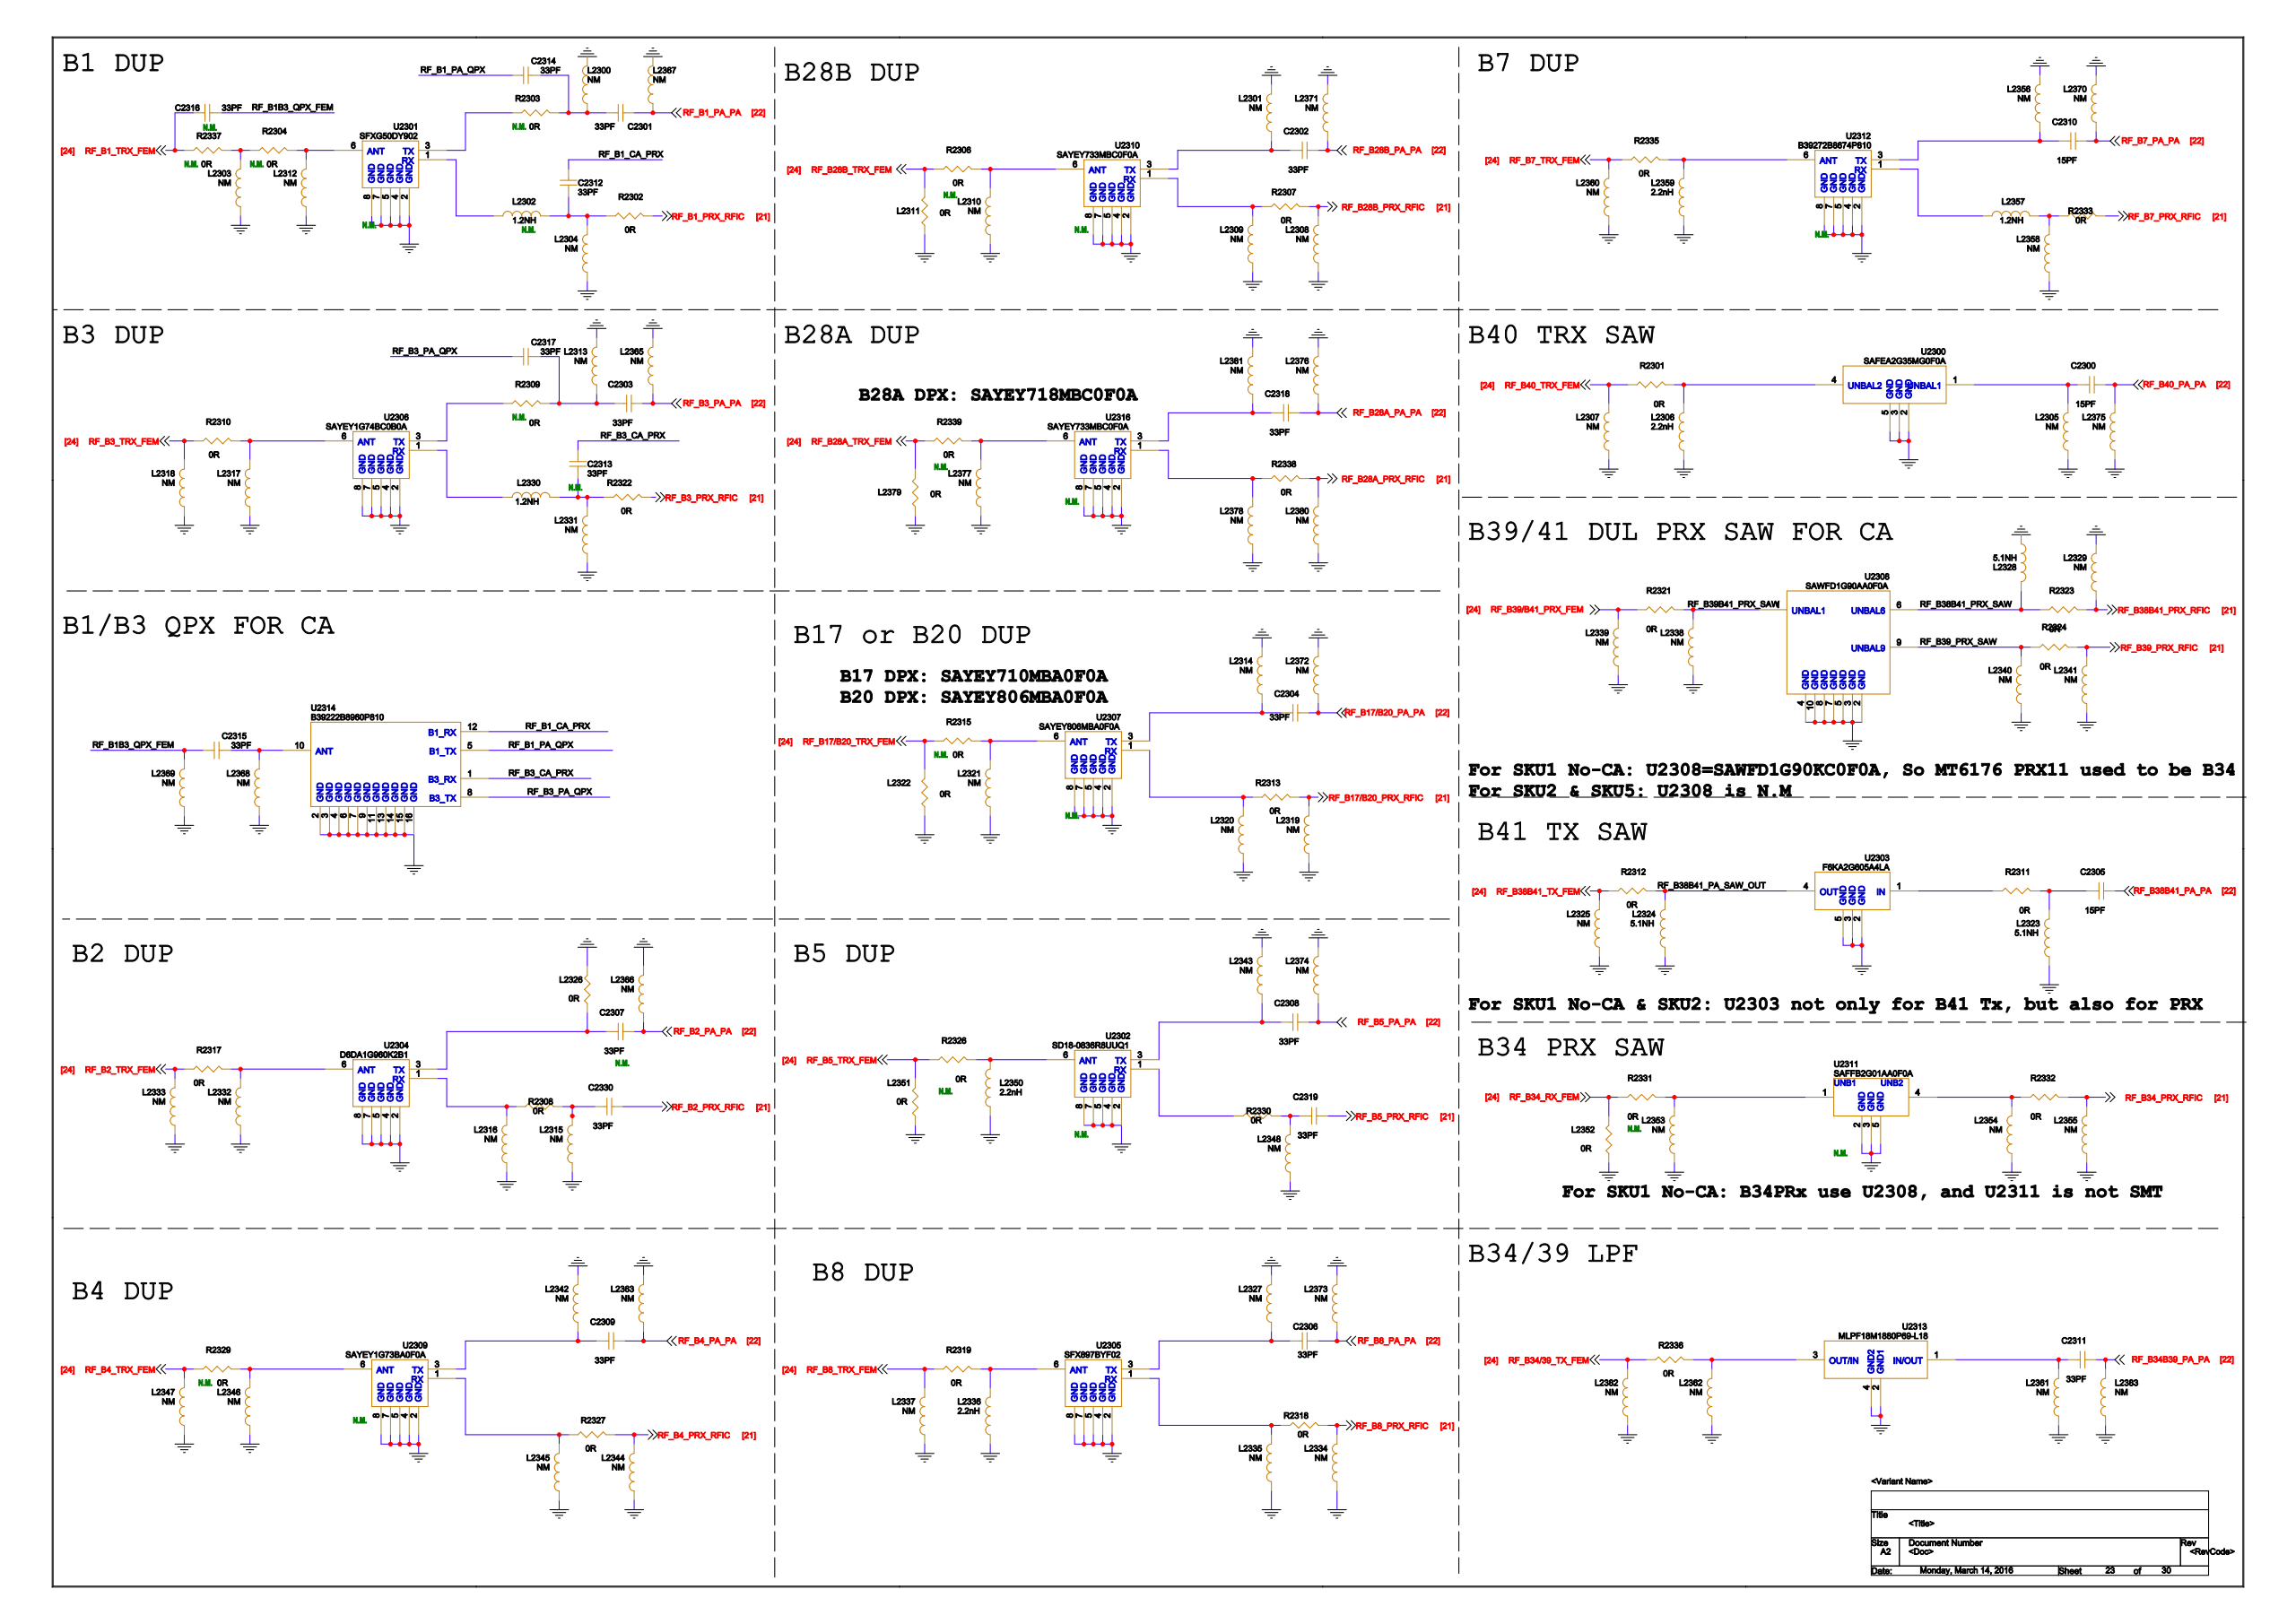Circuit board | Cadence Allegro | 1088 parts | 793 nets | one sheet of the schematic
Parts on this sheet (reference | value | footprint):
C2300 | 15PF | C0201
C2301 | 33PF | C0201
C2302 | 33PF | C0201
C2303 | 33PF | C0201
C2304 | 33PF | C0201
C2305 | 15PF | C0201
C2306 | 33PF | C0201
C2307
C2308 | 33PF | C0201
C2309 | 33PF | C0201
C2310 | 15PF | C0201
C2311 | 33PF | C0201
C2312 | 33PF | C0201
C2313
C2314 | 33PF | C0201
C2315 | 33PF | C0201
C2316
C2317 | 33PF | C0201
C2318 | 33PF | C0201
C2319 | 33PF | C0201
C2330 | 33PF | C0201
L2300 | NM | 0201_NM
L2301 | NM | 0201_NM
L2302
L2303 | NM | 0201_NM
L2304 | NM | 0201_NM
L2305 | NM | 0201_NM
L2306 | 2.2nH | L0201
L2307 | NM | 0201_NM
L2308 | NM | 0201_NM
L2309 | NM | 0201_NM
L2310 | NM | 0201_NM
L2311 | 0R | R0201
L2312 | NM | 0201_NM
L2313 | NM | 0201_NM
L2314 | NM | 0201_NM
L2315 | NM | 0201_NM
L2316 | NM | 0201_NM
L2317 | NM | 0201_NM
L2318 | NM | 0201_NM
L2319 | NM | 0201_NM
L2320 | NM | 0201_NM
L2321 | NM | 0201_NM
L2322 | 0R | R0201
L2323 | 5.1nH | L0201
L2324 | 5.1nH | L0201
L2325 | NM | 0201_NM
L2326 | 0R | R0201
L2327 | NM | 0201_NM
L2328 | 5.1nH | L0201
L2329 | NM | 0201_NM
L2330 | 1.2NH | L0201
L2331 | NM | 0201_NM
L2332 | NM | 0201_NM
L2333 | NM | 0201_NM
L2334 | NM | 0201_NM
L2335 | NM | 0201_NM
L2336 | 2.2nH | L0201
L2337 | NM | 0201_NM
L2338 | NM | 0201_NM
L2339 | NM | 0201_NM
L2340 | NM | 0201_NM
L2341 | NM | 0201_NM
L2342 | NM | 0201_NM
L2343 | NM | 0201_NM
L2344 | NM | 0201_NM
L2345 | NM | 0201_NM
L2346 | NM | 0201_NM
L2347 | NM | 0201_NM
L2348 | NM | 0201_NM
L2350 | 2.2nH | L0201
L2351 | 0R | R0201
L2352 | 0R | R0201
L2353 | NM | 0201_NM
L2354 | NM | 0201_NM
L2355 | NM | 0201_NM
L2356 | NM | 0201_NM
L2357 | 1.2NH | L0201
L2358 | NM | 0201_NM
L2359 | 2.2nH | L0201
L2360 | NM | 0201_NM
L2361 | NM | 0201_NM
L2362 | NM | 0201_NM
L2363 | NM | 0201_NM
L2365 | NM | 0201_NM
L2366 | NM | 0201_NM
L2367 | NM | 0201_NM
L2368 | NM | 0201_NM
L2369 | NM | 0201_NM
L2370 | NM | 0201_NM
L2371 | NM | 0201_NM
L2372 | NM | 0201_NM
L2373 | NM | 0201_NM
L2374 | NM | 0201_NM
L2375 | NM | 0201_NM
L2376 | NM | 0201_NM
L2377 | NM | 0201_NM
L2378 | NM | 0201_NM
L2379 | 0R | R0201
L2380 | NM | 0201_NM
L2381 | NM | 0201_NM
L2382 | NM | 0201_NM
L2383 | NM | 0201_NM
R2301 | 0R | R0201
R2302 | 0R | R0201
R2303
R2304
R2306
R2307 | 0R | R0201
R2308 | 0R | R0201
R2309
R2310 | 0R | R0201
R2311 | 0R | R0201
R2312 | 0R | R0201
R2313 | 0R | R0201
R2315
R2317 | 0R | R0201
R2318 | 0R | R0201
R2319 | 0R | R0201
R2321 | 0R | R0201
R2322 | 0R | R0201
R2323 | 0R | R0201
R2324 | 0R | R0201
R2326
R2327 | 0R | R0201
R2329
R2330 | 0R | R0201
R2331
R2332 | 0R | R0201
R2333 | 0R | R0201
R2335 | 0R | R0201
R2336 | 0R | R0201
R2337
R2338 | 0R | R0201
R2339
U2300 | SAFEA2G35MG0F0A | SAW1411_H0P6_MURATA
U2301
U2302
U2303 | F6KA2G605A4LA | SAW1411_H0P6_TAIYO
U2304 | D6DA1G960K2B1 | D6DA1G960K2B1
U2305 | SFX897BYF02 | DUP1814_H0P73_WISOL
U2306 | SAYEY1G74BC0B0A | DUP1814_H0P7_MURATA
U2307
U2308 | SAWFD1G90AA0F0A | SAW1511_H0P6_MURATA
U2309
U2310
U2311
U2312
U2313 | MLPF18M1880P69-L18 | DEA162025LT-5046E1
U2314 | B39222B8960P810 | B8960
U2316
Nets of these parts (net: part-pin ...):
GND: L2300-1 L2301-1 L2303-2 L2304-2 L2305-2 L2306-2 L2307-2 L2308-2 L2309-2 L2310-2 L2311-2 L2312-2 L2313-1 L2314-1 L2315-2 L2316-2 L2317-2 L2318-2 L2319-2 L2320-2 L2321-2 L2322-2 L2323-2 L2324-2 L2325-2 L2326-1 L2327-1 L2328-1 L2329-1 L2331-2 L2332-2 L2333-2 L2334-2 L2335-2 L2336-2 L2337-2 L2338-2 L2339-2 L2340-2 L2341-2 L2342-1 L2343-1 L2344-2 L2345-2 L2346-2 L2347-2 L2348-2 L2350-2 L2351-2 L2352-1 L2353-2 L2354-2 L2355-2 L2356-1 L2358-2 L2359-2 L2360-2 L2361-2 L2362-2 L2363-1 L2365-1 L2366-1 L2367-1 L2368-2 L2369-2 L2370-1 L2371-1 L2372-1 L2373-1 L2374-1 L2375-2 L2376-1 L2377-2 L2378-2 L2379-2 L2380-2 L2381-1 L2382-2 L2383-2 U2300-2 U2300-3 U2300-5 U2301-2 U2301-4 U2301-5 U2301-7 U2301-8 U2302-2 U2302-4 U2302-5 U2302-7 U2302-8 U2303-2 U2303-3 U2303-5 U2304-2 U2304-4 U2304-5 U2304-7 U2304-8 U2305-2 U2305-4 U2305-5 U2305-7 U2305-8 U2306-2 U2306-4 U2306-5 U2306-7 U2306-8 U2307-2 U2307-4 U2307-5 U2307-7 U2307-8 U2308-2 U2308-3 U2308-4 U2308-5 U2308-7 U2308-8 U2308-10 U2309-2 U2309-4 U2309-5 U2309-7 U2309-8 U2310-2 U2310-4 U2310-5 U2310-7 U2310-8 U2311-2 U2311-3 U2311-5 U2312-2 U2312-4 U2312-5 U2312-7 U2312-8 U2313-2 U2313-4 U2314-2 U2314-3 U2314-4 U2314-6 U2314-7 U2314-9 U2314-11 U2314-13 U2314-14 U2314-15 U2314-16 U2316-2 U2316-4 U2316-5 U2316-7 U2316-8
N33393537: C2305-2 L2323-1 R2311-1
RF_B38B41_PA_SAW_OUT: L2324-1 R2312-1 U2303-4
RF_B38B41_PRX_SAW: L2328-2 R2323-1 U2308-6
N33354934: C2315-2 L2368-1 U2314-10
RF_B1_CA_PRX: C2312-1 U2314-12
RF_B1_PA_QPX: C2314-1 U2314-5
RF_B3_CA_PRX: C2313-1 U2314-1
RF_B3_PA_QPX: C2317-1 U2314-8
N31341559: L2312-1 R2304-1 U2301-6
N32732365: L2302-2 U2301-1
N32732795: R2303-2 U2301-3
N31346744: L2350-1 R2326-1 U2302-6
N33528447: R2330-2 U2302-1
N31346795: C2308-2 L2343-2 U2302-3
N33800339: R2311-2 U2303-1
N33353657: L2332-1 R2317-1 U2304-6
N33353524: L2316-1 R2308-2 U2304-1
N33353528: C2307-2 L2326-2 U2304-3
N33342704: L2336-1 R2319-1 U2305-6
N33342702: L2335-1 R2318-2 U2305-1
N33342522: C2306-2 L2327-2 U2305-3
N31342053: L2317-1 R2310-1 U2306-6
N32730723: L2330-2 U2306-1
N31342005: R2309-2 U2306-3
N33343559: L2321-1 R2315-1 U2307-6
N33343569: L2320-1 R2313-2 U2307-1
N33343567: C2304-2 L2314-2 U2307-3
N33351536: L2346-1 R2329-1 U2309-6
N33351548: L2345-1 R2327-2 U2309-1
N33351497: C2309-2 L2342-2 U2309-3
N31343210: L2310-1 R2306-1 U2310-6
N31343263: L2309-1 R2307-2 U2310-1
N31343162: C2302-2 L2301-2 U2310-3
N33344262: L2377-1 R2339-1 U2316-6
N33344114: L2378-1 R2338-2 U2316-1
N33344260: C2318-2 L2381-2 U2316-3
N33357424: L2359-1 R2335-1 U2312-6
N33357422: L2357-2 U2312-1
N33357352: C2310-2 L2356-2 U2312-3
N33355727: C2311-2 L2361-1 U2313-1
N33355731: L2362-1 R2336-1 U2313-3
RF_B34B39_PA_PA: C2311-1 L2383-1
RF_B28A_PA_PA: C2318-1 L2376-2
RF_B7_PA_PA: C2310-1 L2370-2
RF_B40_PA_PA: C2300-1 L2375-1
RF_B38B41_PA_PA: C2305-1
RF_B5_PA_PA: C2308-1 L2374-2
RF_B8_PA_PA: C2306-1 L2373-2
RF_B17/B20_PA_PA: C2304-1 L2372-2
RF_B2_PA_PA: C2307-1 L2366-2
RF_B3_PA_PA: C2303-1 L2365-2
RF_B1_PA_PA: C2301-1 L2367-2
RF_B28B_PA_PA: C2302-1 L2371-2
RF_B4_PA_PA: C2309-1 L2363-2
RF_B1_TRX_FEM: C2316-1 R2337-2
RF_B8_TRX_FEM: L2337-1 R2319-2
RF_B4_TRX_FEM: L2347-1 R2329-2
RF_B28B_TRX_FEM: L2311-1 R2306-2
RF_B17/B20_TRX_FEM: L2322-1 R2315-2
RF_B5_TRX_FEM: L2351-1 R2326-2
RF_B7_TRX_FEM: L2360-1 R2335-2
RF_B3_TRX_FEM: L2318-1 R2310-2
RF_B40_TRX_FEM: L2307-1 R2301-2
RF_B34/39_TX_FEM: L2382-1 R2336-2
RF_B2_TRX_FEM: L2333-1 R2317-2
RF_B38B41_TX_FEM: L2325-1 R2312-2
RF_B39/B41_PRX_FEM: L2339-1 R2321-1
RF_B2_PRX_RFIC: C2330-1
N35610796: C2330-2 L2315-1 R2308-1
N31341725: C2301-2 C2314-2 L2300-2 R2303-1
N31342104: C2303-2 C2317-2 L2313-2 R2309-1
N31341753: C2312-2 L2302-1 L2304-1 R2302-2
N31342108: C2313-2 L2330-1 L2331-1 R2322-2
RF_B1B3_QPX_FEM: C2315-1 C2316-2 L2369-1
RF_B5_PRX_RFIC: C2319-1
N31346807: C2319-2 L2348-1 R2330-1
N33356442: C2300-2 L2305-1 U2300-1
N31341569: L2303-1 R2304-2 R2337-1
RF_B28B_PRX_RFIC: L2308-1 R2307-1
RF_B17/B20_PRX_RFIC: L2319-1 R2313-1
RF_B38B41_PRX_RFIC: L2329-2 R2323-2
RF_B8_PRX_RFIC: L2334-1 R2318-1
RF_B39B41_PRX_SAW: L2338-1 R2321-2 U2308-1
RF_B39_PRX_SAW: L2340-1 R2324-1 U2308-9
RF_B39_PRX_RFIC: L2341-1 R2324-2
RF_B4_PRX_RFIC: L2344-1 R2327-1
N31370321: L2353-1 R2331-2 U2311-1
N33122945: L2354-1 R2332-1 U2311-4
RF_B34_PRX_RFIC: L2355-1 R2332-2
N33357412: L2357-1 L2358-1 R2333-2
RF_B28A_PRX_RFIC: L2380-1 R2338-1
N33356446: L2306-1 R2301-1 U2300-4
RF_B7_PRX_RFIC: R2333-1
RF_B1_PRX_RFIC: R2302-1
RF_B3_PRX_RFIC: R2322-1
RF_B34_RX_FEM: L2352-2 R2331-1
RF_B28A_TRX_FEM: L2379-1 R2339-2